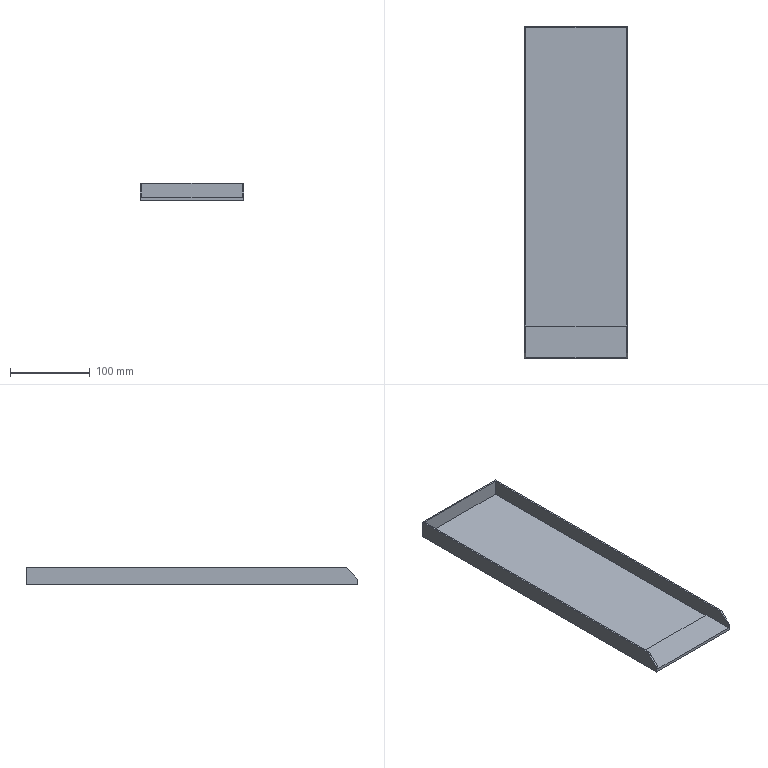Part | NX | features solid 2 | 1 solid | 14 faces | box 130 x 417 x 22 mm | volume 156450 mm3 | plane 14
STEP:
#1=CARTESIAN_POINT('',(-590.,-450.,-300.));
#2=VERTEX_POINT('',#1);
#3=CARTESIAN_POINT('',(-590.,-48.,-300.));
#4=VERTEX_POINT('',#3);
#5=CARTESIAN_POINT('',(-590.,100.,-300.));
#6=DIRECTION('',(0.,-1.,0.));
#7=VECTOR('',#6,1000.);
#8=LINE('',#5,#7);
#9=EDGE_CURVE('',#2,#4,#8,.F.);
#10=ORIENTED_EDGE('',*,*,#9,.F.);
#11=CARTESIAN_POINT('',(-590.,-465.,-315.));
#12=VERTEX_POINT('',#11);
#13=CARTESIAN_POINT('',(-590.,-465.,-315.));
#14=DIRECTION('',(0.,-0.7071,-0.7071));
#15=VECTOR('',#14,1000.);
#16=LINE('',#13,#15);
#17=EDGE_CURVE('',#2,#12,#16,.T.);
#18=ORIENTED_EDGE('',*,*,#17,.T.);
#19=CARTESIAN_POINT('',(-590.,-465.,-322.));
#20=VERTEX_POINT('',#19);
#21=CARTESIAN_POINT('',(-590.,-465.,-320.));
#22=DIRECTION('',(0.,0.,-1.));
#23=VECTOR('',#22,1000.);
#24=LINE('',#21,#23);
#25=EDGE_CURVE('',#12,#20,#24,.T.);
#26=ORIENTED_EDGE('',*,*,#25,.T.);
#27=CARTESIAN_POINT('',(-590.,-48.,-322.));
#28=VERTEX_POINT('',#27);
#29=CARTESIAN_POINT('',(-590.,-15.,-322.));
#30=DIRECTION('',(0.,-1.,0.));
#31=VECTOR('',#30,1000.);
#32=LINE('',#29,#31);
#33=EDGE_CURVE('',#20,#28,#32,.F.);
#34=ORIENTED_EDGE('',*,*,#33,.T.);
#35=CARTESIAN_POINT('',(-590.,-48.,-320.));
#36=DIRECTION('',(0.,0.,-1.));
#37=VECTOR('',#36,1000.);
#38=LINE('',#35,#37);
#39=EDGE_CURVE('',#4,#28,#38,.T.);
#40=ORIENTED_EDGE('',*,*,#39,.F.);
#41=EDGE_LOOP('',(#10,#18,#26,#34,#40));
#42=FACE_BOUND('',#41,.T.);
#43=CARTESIAN_POINT('',(-590.,-15.,-320.));
#44=DIRECTION('',(-1.,0.,0.));
#45=DIRECTION('',(0.,0.,1.));
#46=AXIS2_PLACEMENT_3D('',#43,#44,#45);
#47=PLANE('',#46);
#48=ADVANCED_FACE('',(#42),#47,.F.);
#49=ORIENTED_EDGE('',*,*,#25,.F.);
#50=CARTESIAN_POINT('',(-592.,-465.,-315.));
#51=VERTEX_POINT('',#50);
#52=CARTESIAN_POINT('',(-1120.,-465.,-315.));
#53=DIRECTION('',(-1.,0.,0.));
#54=VECTOR('',#53,1000.);
#55=LINE('',#52,#54);
#56=EDGE_CURVE('',#12,#51,#55,.T.);
#57=ORIENTED_EDGE('',*,*,#56,.T.);
#58=CARTESIAN_POINT('',(-592.,-465.,-318.));
#59=VERTEX_POINT('',#58);
#60=CARTESIAN_POINT('',(-592.,-465.,-320.));
#61=DIRECTION('',(0.,0.,-1.));
#62=VECTOR('',#61,1000.);
#63=LINE('',#60,#62);
#64=EDGE_CURVE('',#51,#59,#63,.T.);
#65=ORIENTED_EDGE('',*,*,#64,.T.);
#66=CARTESIAN_POINT('',(-718.,-465.,-318.));
#67=VERTEX_POINT('',#66);
#68=CARTESIAN_POINT('',(-693.,-465.,-318.));
#69=DIRECTION('',(-1.,0.,0.));
#70=VECTOR('',#69,1000.);
#71=LINE('',#68,#70);
#72=EDGE_CURVE('',#67,#59,#71,.F.);
#73=ORIENTED_EDGE('',*,*,#72,.F.);
#74=CARTESIAN_POINT('',(-718.,-465.,-315.));
#75=VERTEX_POINT('',#74);
#76=CARTESIAN_POINT('',(-718.,-465.,-320.));
#77=DIRECTION('',(0.,0.,-1.));
#78=VECTOR('',#77,1000.);
#79=LINE('',#76,#78);
#80=EDGE_CURVE('',#75,#67,#79,.T.);
#81=ORIENTED_EDGE('',*,*,#80,.F.);
#82=CARTESIAN_POINT('',(-720.,-465.,-315.));
#83=VERTEX_POINT('',#82);
#84=CARTESIAN_POINT('',(-1120.,-465.,-315.));
#85=DIRECTION('',(-1.,0.,0.));
#86=VECTOR('',#85,1000.);
#87=LINE('',#84,#86);
#88=EDGE_CURVE('',#75,#83,#87,.T.);
#89=ORIENTED_EDGE('',*,*,#88,.T.);
#90=CARTESIAN_POINT('',(-720.,-465.,-322.));
#91=VERTEX_POINT('',#90);
#92=CARTESIAN_POINT('',(-720.,-465.,-320.));
#93=DIRECTION('',(0.,0.,-1.));
#94=VECTOR('',#93,1000.);
#95=LINE('',#92,#94);
#96=EDGE_CURVE('',#83,#91,#95,.T.);
#97=ORIENTED_EDGE('',*,*,#96,.T.);
#98=CARTESIAN_POINT('',(-1120.,-465.,-322.));
#99=DIRECTION('',(1.,0.,0.));
#100=VECTOR('',#99,1000.);
#101=LINE('',#98,#100);
#102=EDGE_CURVE('',#91,#20,#101,.T.);
#103=ORIENTED_EDGE('',*,*,#102,.T.);
#104=EDGE_LOOP('',(#49,#57,#65,#73,#81,#89,#97,#103));
#105=FACE_BOUND('',#104,.T.);
#106=CARTESIAN_POINT('',(-1120.,-465.,-320.));
#107=DIRECTION('',(0.,1.,0.));
#108=DIRECTION('',(0.,0.,1.));
#109=AXIS2_PLACEMENT_3D('',#106,#107,#108);
#110=PLANE('',#109);
#111=ADVANCED_FACE('',(#105),#110,.F.);
#112=ORIENTED_EDGE('',*,*,#96,.F.);
#113=CARTESIAN_POINT('',(-720.,-450.,-300.));
#114=VERTEX_POINT('',#113);
#115=CARTESIAN_POINT('',(-720.,-450.,-300.));
#116=DIRECTION('',(0.,0.7071,0.7071));
#117=VECTOR('',#116,1000.);
#118=LINE('',#115,#117);
#119=EDGE_CURVE('',#83,#114,#118,.T.);
#120=ORIENTED_EDGE('',*,*,#119,.T.);
#121=CARTESIAN_POINT('',(-720.,-48.,-300.));
#122=VERTEX_POINT('',#121);
#123=CARTESIAN_POINT('',(-720.,580.,-300.));
#124=DIRECTION('',(0.,-1.,0.));
#125=VECTOR('',#124,1000.);
#126=LINE('',#123,#125);
#127=EDGE_CURVE('',#114,#122,#126,.F.);
#128=ORIENTED_EDGE('',*,*,#127,.T.);
#129=CARTESIAN_POINT('',(-720.,-48.,-322.));
#130=VERTEX_POINT('',#129);
#131=CARTESIAN_POINT('',(-720.,-48.,-320.));
#132=DIRECTION('',(0.,0.,-1.));
#133=VECTOR('',#132,1000.);
#134=LINE('',#131,#133);
#135=EDGE_CURVE('',#122,#130,#134,.T.);
#136=ORIENTED_EDGE('',*,*,#135,.T.);
#137=CARTESIAN_POINT('',(-720.,580.,-322.));
#138=DIRECTION('',(0.,1.,0.));
#139=VECTOR('',#138,1000.);
#140=LINE('',#137,#139);
#141=EDGE_CURVE('',#130,#91,#140,.F.);
#142=ORIENTED_EDGE('',*,*,#141,.T.);
#143=EDGE_LOOP('',(#112,#120,#128,#136,#142));
#144=FACE_BOUND('',#143,.T.);
#145=CARTESIAN_POINT('',(-720.,580.,-320.));
#146=DIRECTION('',(1.,0.,0.));
#147=DIRECTION('',(0.,0.,-1.));
#148=AXIS2_PLACEMENT_3D('',#145,#146,#147);
#149=PLANE('',#148);
#150=ADVANCED_FACE('',(#144),#149,.F.);
#151=CARTESIAN_POINT('',(-718.,-425.,-320.));
#152=VERTEX_POINT('',#151);
#153=CARTESIAN_POINT('',(-592.,-425.,-320.));
#154=VERTEX_POINT('',#153);
#155=CARTESIAN_POINT('',(-693.,-425.,-320.));
#156=DIRECTION('',(1.,0.,0.));
#157=VECTOR('',#156,1000.);
#158=LINE('',#155,#157);
#159=EDGE_CURVE('',#152,#154,#158,.T.);
#160=ORIENTED_EDGE('',*,*,#159,.T.);
#161=CARTESIAN_POINT('',(-592.,-50.,-320.));
#162=VERTEX_POINT('',#161);
#163=CARTESIAN_POINT('',(-592.,-70.,-320.));
#164=DIRECTION('',(0.,1.,0.));
#165=VECTOR('',#164,1000.);
#166=LINE('',#163,#165);
#167=EDGE_CURVE('',#162,#154,#166,.F.);
#168=ORIENTED_EDGE('',*,*,#167,.F.);
#169=CARTESIAN_POINT('',(-718.,-50.,-320.));
#170=VERTEX_POINT('',#169);
#171=CARTESIAN_POINT('',(-590.,-50.,-320.));
#172=DIRECTION('',(1.,0.,0.));
#173=VECTOR('',#172,1000.);
#174=LINE('',#171,#173);
#175=EDGE_CURVE('',#162,#170,#174,.F.);
#176=ORIENTED_EDGE('',*,*,#175,.T.);
#177=CARTESIAN_POINT('',(-718.,-70.,-320.));
#178=DIRECTION('',(0.,-1.,0.));
#179=VECTOR('',#178,1000.);
#180=LINE('',#177,#179);
#181=EDGE_CURVE('',#152,#170,#180,.F.);
#182=ORIENTED_EDGE('',*,*,#181,.F.);
#183=EDGE_LOOP('',(#160,#168,#176,#182));
#184=FACE_BOUND('',#183,.T.);
#185=CARTESIAN_POINT('',(-560.,-70.,-320.));
#186=DIRECTION('',(0.,0.,-1.));
#187=DIRECTION('',(-1.,0.,0.));
#188=AXIS2_PLACEMENT_3D('',#185,#186,#187);
#189=PLANE('',#188);
#190=ADVANCED_FACE('',(#184),#189,.F.);
#191=ORIENTED_EDGE('',*,*,#102,.F.);
#192=ORIENTED_EDGE('',*,*,#141,.F.);
#193=CARTESIAN_POINT('',(-590.,-48.,-322.));
#194=DIRECTION('',(1.,0.,0.));
#195=VECTOR('',#194,1000.);
#196=LINE('',#193,#195);
#197=EDGE_CURVE('',#28,#130,#196,.F.);
#198=ORIENTED_EDGE('',*,*,#197,.F.);
#199=ORIENTED_EDGE('',*,*,#33,.F.);
#200=EDGE_LOOP('',(#191,#192,#198,#199));
#201=FACE_BOUND('',#200,.T.);
#202=CARTESIAN_POINT('',(-560.,-70.,-322.));
#203=DIRECTION('',(0.,0.,-1.));
#204=DIRECTION('',(-1.,0.,0.));
#205=AXIS2_PLACEMENT_3D('',#202,#203,#204);
#206=PLANE('',#205);
#207=ADVANCED_FACE('',(#201),#206,.T.);
#208=CARTESIAN_POINT('',(-592.,-50.,-300.));
#209=VERTEX_POINT('',#208);
#210=CARTESIAN_POINT('',(-592.,-50.,-320.));
#211=DIRECTION('',(0.,0.,-1.));
#212=VECTOR('',#211,1000.);
#213=LINE('',#210,#212);
#214=EDGE_CURVE('',#209,#162,#213,.T.);
#215=ORIENTED_EDGE('',*,*,#214,.F.);
#216=CARTESIAN_POINT('',(-718.,-50.,-300.));
#217=VERTEX_POINT('',#216);
#218=CARTESIAN_POINT('',(-590.,-50.,-300.));
#219=DIRECTION('',(1.,0.,0.));
#220=VECTOR('',#219,1000.);
#221=LINE('',#218,#220);
#222=EDGE_CURVE('',#209,#217,#221,.F.);
#223=ORIENTED_EDGE('',*,*,#222,.T.);
#224=CARTESIAN_POINT('',(-718.,-50.,-320.));
#225=DIRECTION('',(0.,0.,-1.));
#226=VECTOR('',#225,1000.);
#227=LINE('',#224,#226);
#228=EDGE_CURVE('',#217,#170,#227,.T.);
#229=ORIENTED_EDGE('',*,*,#228,.T.);
#230=ORIENTED_EDGE('',*,*,#175,.F.);
#231=EDGE_LOOP('',(#215,#223,#229,#230));
#232=FACE_BOUND('',#231,.T.);
#233=CARTESIAN_POINT('',(-590.,-50.,-320.));
#234=DIRECTION('',(0.,-1.,0.));
#235=DIRECTION('',(0.,0.,-1.));
#236=AXIS2_PLACEMENT_3D('',#233,#234,#235);
#237=PLANE('',#236);
#238=ADVANCED_FACE('',(#232),#237,.T.);
#239=CARTESIAN_POINT('',(-592.,-450.,-300.));
#240=VERTEX_POINT('',#239);
#241=CARTESIAN_POINT('',(-592.,-15.,-300.));
#242=DIRECTION('',(0.,1.,0.));
#243=VECTOR('',#242,1000.);
#244=LINE('',#241,#243);
#245=EDGE_CURVE('',#240,#209,#244,.T.);
#246=ORIENTED_EDGE('',*,*,#245,.F.);
#247=CARTESIAN_POINT('',(-590.,-450.,-300.));
#248=DIRECTION('',(-1.,0.,0.));
#249=VECTOR('',#248,1000.);
#250=LINE('',#247,#249);
#251=EDGE_CURVE('',#240,#2,#250,.F.);
#252=ORIENTED_EDGE('',*,*,#251,.T.);
#253=ORIENTED_EDGE('',*,*,#9,.T.);
#254=CARTESIAN_POINT('',(-590.,-48.,-300.));
#255=DIRECTION('',(1.,0.,0.));
#256=VECTOR('',#255,1000.);
#257=LINE('',#254,#256);
#258=EDGE_CURVE('',#4,#122,#257,.F.);
#259=ORIENTED_EDGE('',*,*,#258,.T.);
#260=ORIENTED_EDGE('',*,*,#127,.F.);
#261=CARTESIAN_POINT('',(-718.,-450.,-300.));
#262=VERTEX_POINT('',#261);
#263=CARTESIAN_POINT('',(-590.,-450.,-300.));
#264=DIRECTION('',(-1.,0.,0.));
#265=VECTOR('',#264,1000.);
#266=LINE('',#263,#265);
#267=EDGE_CURVE('',#114,#262,#266,.F.);
#268=ORIENTED_EDGE('',*,*,#267,.T.);
#269=CARTESIAN_POINT('',(-718.,-15.,-300.));
#270=DIRECTION('',(0.,1.,0.));
#271=VECTOR('',#270,1000.);
#272=LINE('',#269,#271);
#273=EDGE_CURVE('',#217,#262,#272,.F.);
#274=ORIENTED_EDGE('',*,*,#273,.F.);
#275=ORIENTED_EDGE('',*,*,#222,.F.);
#276=EDGE_LOOP('',(#246,#252,#253,#259,#260,#268,#274,#275));
#277=FACE_BOUND('',#276,.T.);
#278=CARTESIAN_POINT('',(-590.,-15.,-300.));
#279=DIRECTION('',(0.,0.,1.));
#280=DIRECTION('',(1.,0.,0.));
#281=AXIS2_PLACEMENT_3D('',#278,#279,#280);
#282=PLANE('',#281);
#283=ADVANCED_FACE('',(#277),#282,.T.);
#284=ORIENTED_EDGE('',*,*,#197,.T.);
#285=ORIENTED_EDGE('',*,*,#135,.F.);
#286=ORIENTED_EDGE('',*,*,#258,.F.);
#287=ORIENTED_EDGE('',*,*,#39,.T.);
#288=EDGE_LOOP('',(#284,#285,#286,#287));
#289=FACE_BOUND('',#288,.T.);
#290=CARTESIAN_POINT('',(-590.,-48.,-320.));
#291=DIRECTION('',(0.,-1.,0.));
#292=DIRECTION('',(0.,0.,-1.));
#293=AXIS2_PLACEMENT_3D('',#290,#291,#292);
#294=PLANE('',#293);
#295=ADVANCED_FACE('',(#289),#294,.F.);
#296=ORIENTED_EDGE('',*,*,#273,.T.);
#297=CARTESIAN_POINT('',(-718.,55.,205.));
#298=DIRECTION('',(0.,-0.7071,-0.7071));
#299=VECTOR('',#298,1000.);
#300=LINE('',#297,#299);
#301=EDGE_CURVE('',#262,#75,#300,.T.);
#302=ORIENTED_EDGE('',*,*,#301,.T.);
#303=ORIENTED_EDGE('',*,*,#80,.T.);
#304=CARTESIAN_POINT('',(-718.,-425.,-318.));
#305=VERTEX_POINT('',#304);
#306=CARTESIAN_POINT('',(-718.,-425.,-318.));
#307=DIRECTION('',(0.,-1.,0.));
#308=VECTOR('',#307,1000.);
#309=LINE('',#306,#308);
#310=EDGE_CURVE('',#305,#67,#309,.T.);
#311=ORIENTED_EDGE('',*,*,#310,.F.);
#312=CARTESIAN_POINT('',(-718.,-425.,-320.));
#313=DIRECTION('',(0.,0.,1.));
#314=VECTOR('',#313,1000.);
#315=LINE('',#312,#314);
#316=EDGE_CURVE('',#152,#305,#315,.T.);
#317=ORIENTED_EDGE('',*,*,#316,.F.);
#318=ORIENTED_EDGE('',*,*,#181,.T.);
#319=ORIENTED_EDGE('',*,*,#228,.F.);
#320=EDGE_LOOP('',(#296,#302,#303,#311,#317,#318,#319));
#321=FACE_BOUND('',#320,.T.);
#322=CARTESIAN_POINT('',(-718.,580.,-320.));
#323=DIRECTION('',(1.,0.,0.));
#324=DIRECTION('',(0.,0.,-1.));
#325=AXIS2_PLACEMENT_3D('',#322,#323,#324);
#326=PLANE('',#325);
#327=ADVANCED_FACE('',(#321),#326,.T.);
#328=ORIENTED_EDGE('',*,*,#64,.F.);
#329=CARTESIAN_POINT('',(-592.,-242.5,-92.5));
#330=DIRECTION('',(0.,0.7071,0.7071));
#331=VECTOR('',#330,1000.);
#332=LINE('',#329,#331);
#333=EDGE_CURVE('',#51,#240,#332,.T.);
#334=ORIENTED_EDGE('',*,*,#333,.T.);
#335=ORIENTED_EDGE('',*,*,#245,.T.);
#336=ORIENTED_EDGE('',*,*,#214,.T.);
#337=ORIENTED_EDGE('',*,*,#167,.T.);
#338=CARTESIAN_POINT('',(-592.,-425.,-318.));
#339=VERTEX_POINT('',#338);
#340=CARTESIAN_POINT('',(-592.,-425.,-320.));
#341=DIRECTION('',(0.,0.,1.));
#342=VECTOR('',#341,1000.);
#343=LINE('',#340,#342);
#344=EDGE_CURVE('',#154,#339,#343,.T.);
#345=ORIENTED_EDGE('',*,*,#344,.T.);
#346=CARTESIAN_POINT('',(-592.,-425.,-318.));
#347=DIRECTION('',(0.,1.,0.));
#348=VECTOR('',#347,1000.);
#349=LINE('',#346,#348);
#350=EDGE_CURVE('',#339,#59,#349,.F.);
#351=ORIENTED_EDGE('',*,*,#350,.T.);
#352=EDGE_LOOP('',(#328,#334,#335,#336,#337,#345,#351));
#353=FACE_BOUND('',#352,.T.);
#354=CARTESIAN_POINT('',(-592.,-15.,-320.));
#355=DIRECTION('',(-1.,0.,0.));
#356=DIRECTION('',(0.,0.,1.));
#357=AXIS2_PLACEMENT_3D('',#354,#355,#356);
#358=PLANE('',#357);
#359=ADVANCED_FACE('',(#353),#358,.T.);
#360=ORIENTED_EDGE('',*,*,#344,.F.);
#361=ORIENTED_EDGE('',*,*,#159,.F.);
#362=ORIENTED_EDGE('',*,*,#316,.T.);
#363=CARTESIAN_POINT('',(-693.,-425.,-318.));
#364=DIRECTION('',(-1.,0.,0.));
#365=VECTOR('',#364,1000.);
#366=LINE('',#363,#365);
#367=EDGE_CURVE('',#305,#339,#366,.F.);
#368=ORIENTED_EDGE('',*,*,#367,.T.);
#369=EDGE_LOOP('',(#360,#361,#362,#368));
#370=FACE_BOUND('',#369,.T.);
#371=CARTESIAN_POINT('',(-693.,-425.,-320.));
#372=DIRECTION('',(0.,1.,0.));
#373=DIRECTION('',(1.,0.,0.));
#374=AXIS2_PLACEMENT_3D('',#371,#372,#373);
#375=PLANE('',#374);
#376=ADVANCED_FACE('',(#370),#375,.T.);
#377=ORIENTED_EDGE('',*,*,#72,.T.);
#378=ORIENTED_EDGE('',*,*,#350,.F.);
#379=ORIENTED_EDGE('',*,*,#367,.F.);
#380=ORIENTED_EDGE('',*,*,#310,.T.);
#381=EDGE_LOOP('',(#377,#378,#379,#380));
#382=FACE_BOUND('',#381,.T.);
#383=CARTESIAN_POINT('',(-693.,-425.,-318.));
#384=DIRECTION('',(0.,0.,-1.));
#385=DIRECTION('',(-1.,0.,0.));
#386=AXIS2_PLACEMENT_3D('',#383,#384,#385);
#387=PLANE('',#386);
#388=ADVANCED_FACE('',(#382),#387,.F.);
#389=ORIENTED_EDGE('',*,*,#119,.F.);
#390=ORIENTED_EDGE('',*,*,#88,.F.);
#391=ORIENTED_EDGE('',*,*,#301,.F.);
#392=ORIENTED_EDGE('',*,*,#267,.F.);
#393=EDGE_LOOP('',(#389,#390,#391,#392));
#394=FACE_BOUND('',#393,.T.);
#395=CARTESIAN_POINT('',(-590.,-450.,-300.));
#396=DIRECTION('',(0.,-0.7071,0.7071));
#397=DIRECTION('',(0.,-0.7071,-0.7071));
#398=AXIS2_PLACEMENT_3D('',#395,#396,#397);
#399=PLANE('',#398);
#400=ADVANCED_FACE('',(#394),#399,.T.);
#401=ORIENTED_EDGE('',*,*,#17,.F.);
#402=ORIENTED_EDGE('',*,*,#251,.F.);
#403=ORIENTED_EDGE('',*,*,#333,.F.);
#404=ORIENTED_EDGE('',*,*,#56,.F.);
#405=EDGE_LOOP('',(#401,#402,#403,#404));
#406=FACE_BOUND('',#405,.T.);
#407=CARTESIAN_POINT('',(-1120.,-465.,-315.));
#408=DIRECTION('',(0.,-0.7071,0.7071));
#409=DIRECTION('',(0.,-0.7071,-0.7071));
#410=AXIS2_PLACEMENT_3D('',#407,#408,#409);
#411=PLANE('',#410);
#412=ADVANCED_FACE('',(#406),#411,.T.);
#413=CLOSED_SHELL('',(#48,#111,#150,#190,#207,#238,#283,#295,#327,#359,#376,#388,#400,#412));
#414=MANIFOLD_SOLID_BREP('',#413);
#415=(LENGTH_UNIT()NAMED_UNIT(*)SI_UNIT(.MILLI.,.METRE.));
#416=UNCERTAINTY_MEASURE_WITH_UNIT(LENGTH_MEASURE(0.00001),#415,'','');
#417=(NAMED_UNIT(*)PLANE_ANGLE_UNIT()SI_UNIT($,.RADIAN.));
#418=(NAMED_UNIT(*)SI_UNIT($,.STERADIAN.)SOLID_ANGLE_UNIT());
#419=(GEOMETRIC_REPRESENTATION_CONTEXT(3)GLOBAL_UNCERTAINTY_ASSIGNED_CONTEXT((#416))GLOBAL_UNIT_ASSIGNED_CONTEXT((#415,#417,#418))REPRESENTATION_CONTEXT('',''));
#420=ADVANCED_BREP_SHAPE_REPRESENTATION('',(#414),#419);